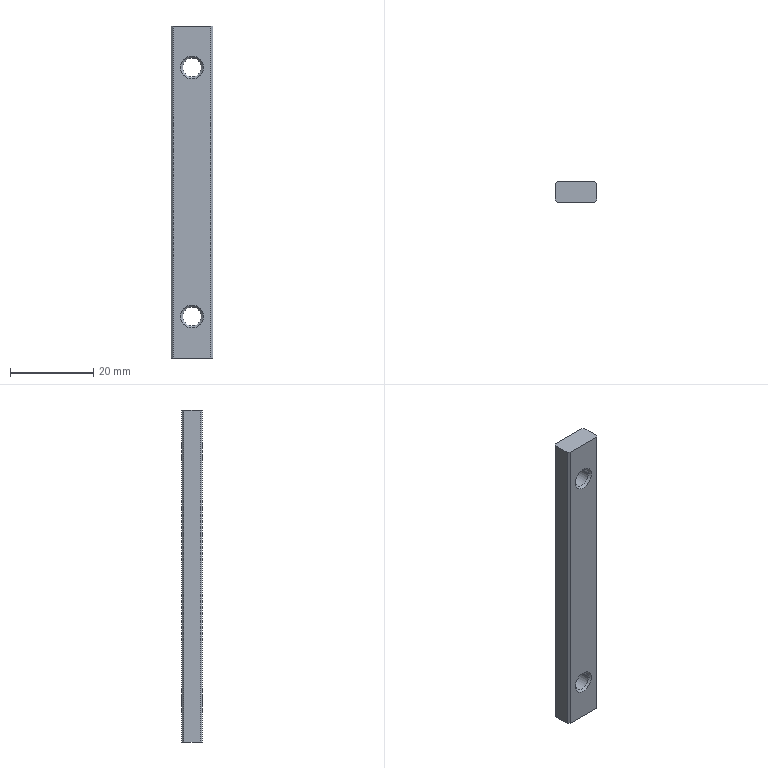Part | NX | 1 solid | 22 faces | box 10 x 5 x 80 mm | volume 3793 mm3 | plane 10 | cone 8 | cylinder 4 | commonest cylinder face diameters 4.5 x4
STEP:
#1=CARTESIAN_POINT('',(0.,2.,40.));
#2=VERTEX_POINT('',#1);
#3=CARTESIAN_POINT('',(0.,-2.,40.));
#4=VERTEX_POINT('',#3);
#5=CARTESIAN_POINT('',(0.,0.,40.));
#6=DIRECTION('',(0.,-1.,0.));
#7=VECTOR('',#6,1000.);
#8=LINE('',#5,#7);
#9=EDGE_CURVE('',#2,#4,#8,.T.);
#10=ORIENTED_EDGE('',*,*,#9,.F.);
#11=CARTESIAN_POINT('',(0.,2.,-40.));
#12=VERTEX_POINT('',#11);
#13=CARTESIAN_POINT('',(0.,2.,0.));
#14=DIRECTION('',(0.,0.,-1.));
#15=VECTOR('',#14,1000.);
#16=LINE('',#13,#15);
#17=EDGE_CURVE('',#2,#12,#16,.T.);
#18=ORIENTED_EDGE('',*,*,#17,.T.);
#19=CARTESIAN_POINT('',(0.,-2.,-40.));
#20=VERTEX_POINT('',#19);
#21=CARTESIAN_POINT('',(0.,0.,-40.));
#22=DIRECTION('',(0.,-1.,0.));
#23=VECTOR('',#22,1000.);
#24=LINE('',#21,#23);
#25=EDGE_CURVE('',#12,#20,#24,.T.);
#26=ORIENTED_EDGE('',*,*,#25,.T.);
#27=CARTESIAN_POINT('',(0.,-2.,0.));
#28=DIRECTION('',(0.,0.,1.));
#29=VECTOR('',#28,1000.);
#30=LINE('',#27,#29);
#31=EDGE_CURVE('',#20,#4,#30,.T.);
#32=ORIENTED_EDGE('',*,*,#31,.T.);
#33=EDGE_LOOP('',(#10,#18,#26,#32));
#34=FACE_BOUND('',#33,.T.);
#35=CARTESIAN_POINT('',(0.,0.,0.));
#36=DIRECTION('',(1.,0.,0.));
#37=DIRECTION('',(0.,1.,0.));
#38=AXIS2_PLACEMENT_3D('',#35,#36,#37);
#39=PLANE('',#38);
#40=ADVANCED_FACE('',(#34),#39,.F.);
#41=CARTESIAN_POINT('',(7.25,2.,-30.));
#42=VERTEX_POINT('',#41);
#43=CARTESIAN_POINT('',(2.75,2.,-30.));
#44=VERTEX_POINT('',#43);
#45=CARTESIAN_POINT('',(5.,2.,-30.));
#46=DIRECTION('',(0.,1.,0.));
#47=DIRECTION('',(1.,0.,0.));
#48=AXIS2_PLACEMENT_3D('',#45,#46,#47);
#49=CIRCLE('',#48,2.25);
#50=EDGE_CURVE('',#42,#44,#49,.T.);
#51=ORIENTED_EDGE('',*,*,#50,.T.);
#52=CARTESIAN_POINT('',(2.75,-2.,-30.));
#53=VERTEX_POINT('',#52);
#54=CARTESIAN_POINT('',(2.75,2.5,-30.));
#55=DIRECTION('',(0.,-1.,0.));
#56=VECTOR('',#55,1000.);
#57=LINE('',#54,#56);
#58=EDGE_CURVE('',#53,#44,#57,.F.);
#59=ORIENTED_EDGE('',*,*,#58,.F.);
#60=CARTESIAN_POINT('',(7.25,-2.,-30.));
#61=VERTEX_POINT('',#60);
#62=CARTESIAN_POINT('',(5.,-2.,-30.));
#63=DIRECTION('',(0.,-1.,0.));
#64=DIRECTION('',(-1.,0.,0.));
#65=AXIS2_PLACEMENT_3D('',#62,#63,#64);
#66=CIRCLE('',#65,2.25);
#67=EDGE_CURVE('',#53,#61,#66,.T.);
#68=ORIENTED_EDGE('',*,*,#67,.T.);
#69=CARTESIAN_POINT('',(7.25,2.5,-30.));
#70=DIRECTION('',(0.,-1.,0.));
#71=VECTOR('',#70,1000.);
#72=LINE('',#69,#71);
#73=EDGE_CURVE('',#61,#42,#72,.F.);
#74=ORIENTED_EDGE('',*,*,#73,.T.);
#75=EDGE_LOOP('',(#51,#59,#68,#74));
#76=FACE_BOUND('',#75,.T.);
#77=CARTESIAN_POINT('',(5.,2.5,-30.));
#78=DIRECTION('',(0.,-1.,0.));
#79=DIRECTION('',(1.,0.,0.));
#80=AXIS2_PLACEMENT_3D('',#77,#78,#79);
#81=CYLINDRICAL_SURFACE('',#80,2.25);
#82=ADVANCED_FACE('',(#76),#81,.F.);
#83=CARTESIAN_POINT('',(0.5,2.5,40.));
#84=VERTEX_POINT('',#83);
#85=CARTESIAN_POINT('',(-2.,0.,40.));
#86=DIRECTION('',(0.7071,0.7071,0.));
#87=VECTOR('',#86,1000.);
#88=LINE('',#85,#87);
#89=EDGE_CURVE('',#2,#84,#88,.T.);
#90=ORIENTED_EDGE('',*,*,#89,.T.);
#91=CARTESIAN_POINT('',(0.5,2.5,-40.));
#92=VERTEX_POINT('',#91);
#93=CARTESIAN_POINT('',(0.5,2.5,0.));
#94=DIRECTION('',(0.,0.,-1.));
#95=VECTOR('',#94,1000.);
#96=LINE('',#93,#95);
#97=EDGE_CURVE('',#84,#92,#96,.T.);
#98=ORIENTED_EDGE('',*,*,#97,.T.);
#99=CARTESIAN_POINT('',(-2.,0.,-40.));
#100=DIRECTION('',(-0.7071,-0.7071,0.));
#101=VECTOR('',#100,1000.);
#102=LINE('',#99,#101);
#103=EDGE_CURVE('',#92,#12,#102,.T.);
#104=ORIENTED_EDGE('',*,*,#103,.T.);
#105=ORIENTED_EDGE('',*,*,#17,.F.);
#106=EDGE_LOOP('',(#90,#98,#104,#105));
#107=FACE_BOUND('',#106,.T.);
#108=CARTESIAN_POINT('',(0.,2.,-40.));
#109=DIRECTION('',(-0.7071,0.7071,0.));
#110=DIRECTION('',(0.,0.,1.));
#111=AXIS2_PLACEMENT_3D('',#108,#109,#110);
#112=PLANE('',#111);
#113=ADVANCED_FACE('',(#107),#112,.T.);
#114=ORIENTED_EDGE('',*,*,#9,.T.);
#115=CARTESIAN_POINT('',(0.5,-2.5,40.));
#116=VERTEX_POINT('',#115);
#117=CARTESIAN_POINT('',(-2.,0.,40.));
#118=DIRECTION('',(-0.7071,0.7071,0.));
#119=VECTOR('',#118,1000.);
#120=LINE('',#117,#119);
#121=EDGE_CURVE('',#116,#4,#120,.T.);
#122=ORIENTED_EDGE('',*,*,#121,.F.);
#123=CARTESIAN_POINT('',(9.5,-2.5,40.));
#124=VERTEX_POINT('',#123);
#125=CARTESIAN_POINT('',(0.,-2.5,40.));
#126=DIRECTION('',(-1.,0.,0.));
#127=VECTOR('',#126,1000.);
#128=LINE('',#125,#127);
#129=EDGE_CURVE('',#124,#116,#128,.T.);
#130=ORIENTED_EDGE('',*,*,#129,.F.);
#131=CARTESIAN_POINT('',(10.,-2.,40.));
#132=VERTEX_POINT('',#131);
#133=CARTESIAN_POINT('',(12.,0.,40.));
#134=DIRECTION('',(0.7071,0.7071,0.));
#135=VECTOR('',#134,1000.);
#136=LINE('',#133,#135);
#137=EDGE_CURVE('',#124,#132,#136,.T.);
#138=ORIENTED_EDGE('',*,*,#137,.T.);
#139=CARTESIAN_POINT('',(10.,2.,40.));
#140=VERTEX_POINT('',#139);
#141=CARTESIAN_POINT('',(10.,0.,40.));
#142=DIRECTION('',(0.,-1.,0.));
#143=VECTOR('',#142,1000.);
#144=LINE('',#141,#143);
#145=EDGE_CURVE('',#140,#132,#144,.T.);
#146=ORIENTED_EDGE('',*,*,#145,.F.);
#147=CARTESIAN_POINT('',(9.5,2.5,40.));
#148=VERTEX_POINT('',#147);
#149=CARTESIAN_POINT('',(12.,0.,40.));
#150=DIRECTION('',(-0.7071,0.7071,0.));
#151=VECTOR('',#150,1000.);
#152=LINE('',#149,#151);
#153=EDGE_CURVE('',#140,#148,#152,.T.);
#154=ORIENTED_EDGE('',*,*,#153,.T.);
#155=CARTESIAN_POINT('',(0.,2.5,40.));
#156=DIRECTION('',(-1.,0.,0.));
#157=VECTOR('',#156,1000.);
#158=LINE('',#155,#157);
#159=EDGE_CURVE('',#148,#84,#158,.T.);
#160=ORIENTED_EDGE('',*,*,#159,.T.);
#161=ORIENTED_EDGE('',*,*,#89,.F.);
#162=EDGE_LOOP('',(#114,#122,#130,#138,#146,#154,#160,#161));
#163=FACE_BOUND('',#162,.T.);
#164=CARTESIAN_POINT('',(0.,2.5,40.));
#165=DIRECTION('',(0.,0.,1.));
#166=DIRECTION('',(1.,0.,0.));
#167=AXIS2_PLACEMENT_3D('',#164,#165,#166);
#168=PLANE('',#167);
#169=ADVANCED_FACE('',(#163),#168,.T.);
#170=CARTESIAN_POINT('',(0.5,-2.5,-40.));
#171=VERTEX_POINT('',#170);
#172=CARTESIAN_POINT('',(-2.,0.,-40.));
#173=DIRECTION('',(-0.7071,0.7071,0.));
#174=VECTOR('',#173,1000.);
#175=LINE('',#172,#174);
#176=EDGE_CURVE('',#171,#20,#175,.T.);
#177=ORIENTED_EDGE('',*,*,#176,.F.);
#178=CARTESIAN_POINT('',(0.5,-2.5,0.));
#179=DIRECTION('',(0.,0.,-1.));
#180=VECTOR('',#179,1000.);
#181=LINE('',#178,#180);
#182=EDGE_CURVE('',#116,#171,#181,.T.);
#183=ORIENTED_EDGE('',*,*,#182,.F.);
#184=ORIENTED_EDGE('',*,*,#121,.T.);
#185=ORIENTED_EDGE('',*,*,#31,.F.);
#186=EDGE_LOOP('',(#177,#183,#184,#185));
#187=FACE_BOUND('',#186,.T.);
#188=CARTESIAN_POINT('',(0.,-2.,39.5));
#189=DIRECTION('',(-0.7071,-0.7071,0.));
#190=DIRECTION('',(-0.7071,0.7071,0.));
#191=AXIS2_PLACEMENT_3D('',#188,#189,#190);
#192=PLANE('',#191);
#193=ADVANCED_FACE('',(#187),#192,.T.);
#194=CARTESIAN_POINT('',(10.,2.,-40.));
#195=VERTEX_POINT('',#194);
#196=CARTESIAN_POINT('',(9.5,2.5,-40.));
#197=VERTEX_POINT('',#196);
#198=CARTESIAN_POINT('',(12.,0.,-40.));
#199=DIRECTION('',(-0.7071,0.7071,0.));
#200=VECTOR('',#199,1000.);
#201=LINE('',#198,#200);
#202=EDGE_CURVE('',#195,#197,#201,.T.);
#203=ORIENTED_EDGE('',*,*,#202,.T.);
#204=CARTESIAN_POINT('',(9.5,2.5,0.));
#205=DIRECTION('',(0.,0.,-1.));
#206=VECTOR('',#205,1000.);
#207=LINE('',#204,#206);
#208=EDGE_CURVE('',#148,#197,#207,.T.);
#209=ORIENTED_EDGE('',*,*,#208,.F.);
#210=ORIENTED_EDGE('',*,*,#153,.F.);
#211=CARTESIAN_POINT('',(10.,2.,0.));
#212=DIRECTION('',(0.,0.,-1.));
#213=VECTOR('',#212,1000.);
#214=LINE('',#211,#213);
#215=EDGE_CURVE('',#140,#195,#214,.T.);
#216=ORIENTED_EDGE('',*,*,#215,.T.);
#217=EDGE_LOOP('',(#203,#209,#210,#216));
#218=FACE_BOUND('',#217,.T.);
#219=CARTESIAN_POINT('',(10.,2.,-40.));
#220=DIRECTION('',(-0.7071,-0.7071,0.));
#221=DIRECTION('',(-0.7071,0.7071,0.));
#222=AXIS2_PLACEMENT_3D('',#219,#220,#221);
#223=PLANE('',#222);
#224=ADVANCED_FACE('',(#218),#223,.F.);
#225=ORIENTED_EDGE('',*,*,#129,.T.);
#226=ORIENTED_EDGE('',*,*,#182,.T.);
#227=CARTESIAN_POINT('',(9.5,-2.5,-40.));
#228=VERTEX_POINT('',#227);
#229=CARTESIAN_POINT('',(0.,-2.5,-40.));
#230=DIRECTION('',(1.,0.,0.));
#231=VECTOR('',#230,1000.);
#232=LINE('',#229,#231);
#233=EDGE_CURVE('',#171,#228,#232,.T.);
#234=ORIENTED_EDGE('',*,*,#233,.T.);
#235=CARTESIAN_POINT('',(9.5,-2.5,0.));
#236=DIRECTION('',(0.,0.,-1.));
#237=VECTOR('',#236,1000.);
#238=LINE('',#235,#237);
#239=EDGE_CURVE('',#124,#228,#238,.T.);
#240=ORIENTED_EDGE('',*,*,#239,.F.);
#241=EDGE_LOOP('',(#225,#226,#234,#240));
#242=FACE_BOUND('',#241,.T.);
#243=CARTESIAN_POINT('',(2.25,-2.5,30.));
#244=VERTEX_POINT('',#243);
#245=CARTESIAN_POINT('',(7.75,-2.5,30.));
#246=VERTEX_POINT('',#245);
#247=CARTESIAN_POINT('',(5.,-2.5,30.));
#248=DIRECTION('',(0.,-1.,0.));
#249=DIRECTION('',(-1.,0.,0.));
#250=AXIS2_PLACEMENT_3D('',#247,#248,#249);
#251=CIRCLE('',#250,2.75);
#252=EDGE_CURVE('',#244,#246,#251,.T.);
#253=ORIENTED_EDGE('',*,*,#252,.F.);
#254=CARTESIAN_POINT('',(5.,-2.5,30.));
#255=DIRECTION('',(0.,-1.,0.));
#256=DIRECTION('',(-1.,0.,0.));
#257=AXIS2_PLACEMENT_3D('',#254,#255,#256);
#258=CIRCLE('',#257,2.75);
#259=EDGE_CURVE('',#246,#244,#258,.T.);
#260=ORIENTED_EDGE('',*,*,#259,.F.);
#261=EDGE_LOOP('',(#253,#260));
#262=FACE_BOUND('',#261,.T.);
#263=CARTESIAN_POINT('',(7.75,-2.5,-30.));
#264=VERTEX_POINT('',#263);
#265=CARTESIAN_POINT('',(2.25,-2.5,-30.));
#266=VERTEX_POINT('',#265);
#267=CARTESIAN_POINT('',(5.,-2.5,-30.));
#268=DIRECTION('',(0.,-1.,0.));
#269=DIRECTION('',(-1.,0.,0.));
#270=AXIS2_PLACEMENT_3D('',#267,#268,#269);
#271=CIRCLE('',#270,2.75);
#272=EDGE_CURVE('',#264,#266,#271,.T.);
#273=ORIENTED_EDGE('',*,*,#272,.F.);
#274=CARTESIAN_POINT('',(5.,-2.5,-30.));
#275=DIRECTION('',(0.,-1.,0.));
#276=DIRECTION('',(-1.,0.,0.));
#277=AXIS2_PLACEMENT_3D('',#274,#275,#276);
#278=CIRCLE('',#277,2.75);
#279=EDGE_CURVE('',#266,#264,#278,.T.);
#280=ORIENTED_EDGE('',*,*,#279,.F.);
#281=EDGE_LOOP('',(#273,#280));
#282=FACE_BOUND('',#281,.T.);
#283=CARTESIAN_POINT('',(0.,-2.5,40.));
#284=DIRECTION('',(0.,-1.,0.));
#285=DIRECTION('',(0.,0.,-1.));
#286=AXIS2_PLACEMENT_3D('',#283,#284,#285);
#287=PLANE('',#286);
#288=ADVANCED_FACE('',(#242,#262,#282),#287,.T.);
#289=ORIENTED_EDGE('',*,*,#137,.F.);
#290=ORIENTED_EDGE('',*,*,#239,.T.);
#291=CARTESIAN_POINT('',(10.,-2.,-40.));
#292=VERTEX_POINT('',#291);
#293=CARTESIAN_POINT('',(12.,0.,-40.));
#294=DIRECTION('',(0.7071,0.7071,0.));
#295=VECTOR('',#294,1000.);
#296=LINE('',#293,#295);
#297=EDGE_CURVE('',#228,#292,#296,.T.);
#298=ORIENTED_EDGE('',*,*,#297,.T.);
#299=CARTESIAN_POINT('',(10.,-2.,0.));
#300=DIRECTION('',(0.,0.,-1.));
#301=VECTOR('',#300,1000.);
#302=LINE('',#299,#301);
#303=EDGE_CURVE('',#132,#292,#302,.T.);
#304=ORIENTED_EDGE('',*,*,#303,.F.);
#305=EDGE_LOOP('',(#289,#290,#298,#304));
#306=FACE_BOUND('',#305,.T.);
#307=CARTESIAN_POINT('',(10.,-2.,40.));
#308=DIRECTION('',(-0.7071,0.7071,0.));
#309=DIRECTION('',(0.,0.,1.));
#310=AXIS2_PLACEMENT_3D('',#307,#308,#309);
#311=PLANE('',#310);
#312=ADVANCED_FACE('',(#306),#311,.F.);
#313=CARTESIAN_POINT('',(10.,0.,-40.));
#314=DIRECTION('',(0.,-1.,0.));
#315=VECTOR('',#314,1000.);
#316=LINE('',#313,#315);
#317=EDGE_CURVE('',#195,#292,#316,.T.);
#318=ORIENTED_EDGE('',*,*,#317,.F.);
#319=ORIENTED_EDGE('',*,*,#215,.F.);
#320=ORIENTED_EDGE('',*,*,#145,.T.);
#321=ORIENTED_EDGE('',*,*,#303,.T.);
#322=EDGE_LOOP('',(#318,#319,#320,#321));
#323=FACE_BOUND('',#322,.T.);
#324=CARTESIAN_POINT('',(10.,0.,0.));
#325=DIRECTION('',(1.,0.,0.));
#326=DIRECTION('',(0.,1.,0.));
#327=AXIS2_PLACEMENT_3D('',#324,#325,#326);
#328=PLANE('',#327);
#329=ADVANCED_FACE('',(#323),#328,.T.);
#330=CARTESIAN_POINT('',(2.75,-2.,30.));
#331=VERTEX_POINT('',#330);
#332=CARTESIAN_POINT('',(7.25,-2.,30.));
#333=VERTEX_POINT('',#332);
#334=CARTESIAN_POINT('',(5.,-2.,30.));
#335=DIRECTION('',(0.,-1.,0.));
#336=DIRECTION('',(-1.,0.,0.));
#337=AXIS2_PLACEMENT_3D('',#334,#335,#336);
#338=CIRCLE('',#337,2.25);
#339=EDGE_CURVE('',#331,#333,#338,.T.);
#340=ORIENTED_EDGE('',*,*,#339,.T.);
#341=CARTESIAN_POINT('',(7.25,2.,30.));
#342=VERTEX_POINT('',#341);
#343=CARTESIAN_POINT('',(7.25,2.5,30.));
#344=DIRECTION('',(0.,-1.,0.));
#345=VECTOR('',#344,1000.);
#346=LINE('',#343,#345);
#347=EDGE_CURVE('',#342,#333,#346,.T.);
#348=ORIENTED_EDGE('',*,*,#347,.F.);
#349=CARTESIAN_POINT('',(2.75,2.,30.));
#350=VERTEX_POINT('',#349);
#351=CARTESIAN_POINT('',(5.,2.,30.));
#352=DIRECTION('',(0.,1.,0.));
#353=DIRECTION('',(1.,0.,0.));
#354=AXIS2_PLACEMENT_3D('',#351,#352,#353);
#355=CIRCLE('',#354,2.25);
#356=EDGE_CURVE('',#342,#350,#355,.T.);
#357=ORIENTED_EDGE('',*,*,#356,.T.);
#358=CARTESIAN_POINT('',(2.75,2.5,30.));
#359=DIRECTION('',(0.,-1.,0.));
#360=VECTOR('',#359,1000.);
#361=LINE('',#358,#360);
#362=EDGE_CURVE('',#350,#331,#361,.T.);
#363=ORIENTED_EDGE('',*,*,#362,.T.);
#364=EDGE_LOOP('',(#340,#348,#357,#363));
#365=FACE_BOUND('',#364,.T.);
#366=CARTESIAN_POINT('',(5.,2.5,30.));
#367=DIRECTION('',(0.,-1.,0.));
#368=DIRECTION('',(1.,0.,0.));
#369=AXIS2_PLACEMENT_3D('',#366,#367,#368);
#370=CYLINDRICAL_SURFACE('',#369,2.25);
#371=ADVANCED_FACE('',(#365),#370,.F.);
#372=CARTESIAN_POINT('',(0.,2.5,-40.));
#373=DIRECTION('',(1.,0.,0.));
#374=VECTOR('',#373,1000.);
#375=LINE('',#372,#374);
#376=EDGE_CURVE('',#92,#197,#375,.T.);
#377=ORIENTED_EDGE('',*,*,#376,.F.);
#378=ORIENTED_EDGE('',*,*,#97,.F.);
#379=ORIENTED_EDGE('',*,*,#159,.F.);
#380=ORIENTED_EDGE('',*,*,#208,.T.);
#381=EDGE_LOOP('',(#377,#378,#379,#380));
#382=FACE_BOUND('',#381,.T.);
#383=CARTESIAN_POINT('',(7.75,2.5,30.));
#384=VERTEX_POINT('',#383);
#385=CARTESIAN_POINT('',(2.25,2.5,30.));
#386=VERTEX_POINT('',#385);
#387=CARTESIAN_POINT('',(5.,2.5,30.));
#388=DIRECTION('',(0.,1.,0.));
#389=DIRECTION('',(1.,0.,0.));
#390=AXIS2_PLACEMENT_3D('',#387,#388,#389);
#391=CIRCLE('',#390,2.75);
#392=EDGE_CURVE('',#384,#386,#391,.T.);
#393=ORIENTED_EDGE('',*,*,#392,.F.);
#394=CARTESIAN_POINT('',(5.,2.5,30.));
#395=DIRECTION('',(0.,1.,0.));
#396=DIRECTION('',(1.,0.,0.));
#397=AXIS2_PLACEMENT_3D('',#394,#395,#396);
#398=CIRCLE('',#397,2.75);
#399=EDGE_CURVE('',#386,#384,#398,.T.);
#400=ORIENTED_EDGE('',*,*,#399,.F.);
#401=EDGE_LOOP('',(#393,#400));
#402=FACE_BOUND('',#401,.T.);
#403=CARTESIAN_POINT('',(2.25,2.5,-30.));
#404=VERTEX_POINT('',#403);
#405=CARTESIAN_POINT('',(7.75,2.5,-30.));
#406=VERTEX_POINT('',#405);
#407=CARTESIAN_POINT('',(5.,2.5,-30.));
#408=DIRECTION('',(0.,1.,0.));
#409=DIRECTION('',(1.,0.,0.));
#410=AXIS2_PLACEMENT_3D('',#407,#408,#409);
#411=CIRCLE('',#410,2.75);
#412=EDGE_CURVE('',#404,#406,#411,.T.);
#413=ORIENTED_EDGE('',*,*,#412,.F.);
#414=CARTESIAN_POINT('',(5.,2.5,-30.));
#415=DIRECTION('',(0.,1.,0.));
#416=DIRECTION('',(1.,0.,0.));
#417=AXIS2_PLACEMENT_3D('',#414,#415,#416);
#418=CIRCLE('',#417,2.75);
#419=EDGE_CURVE('',#406,#404,#418,.T.);
#420=ORIENTED_EDGE('',*,*,#419,.F.);
#421=EDGE_LOOP('',(#413,#420));
#422=FACE_BOUND('',#421,.T.);
#423=CARTESIAN_POINT('',(0.,2.5,-40.));
#424=DIRECTION('',(0.,1.,0.));
#425=DIRECTION('',(1.,0.,0.));
#426=AXIS2_PLACEMENT_3D('',#423,#424,#425);
#427=PLANE('',#426);
#428=ADVANCED_FACE('',(#382,#402,#422),#427,.T.);
#429=ORIENTED_EDGE('',*,*,#176,.T.);
#430=ORIENTED_EDGE('',*,*,#25,.F.);
#431=ORIENTED_EDGE('',*,*,#103,.F.);
#432=ORIENTED_EDGE('',*,*,#376,.T.);
#433=ORIENTED_EDGE('',*,*,#202,.F.);
#434=ORIENTED_EDGE('',*,*,#317,.T.);
#435=ORIENTED_EDGE('',*,*,#297,.F.);
#436=ORIENTED_EDGE('',*,*,#233,.F.);
#437=EDGE_LOOP('',(#429,#430,#431,#432,#433,#434,#435,#436));
#438=FACE_BOUND('',#437,.T.);
#439=CARTESIAN_POINT('',(0.,-2.5,-40.));
#440=DIRECTION('',(0.,0.,-1.));
#441=DIRECTION('',(0.,-1.,0.));
#442=AXIS2_PLACEMENT_3D('',#439,#440,#441);
#443=PLANE('',#442);
#444=ADVANCED_FACE('',(#438),#443,.T.);
#445=ORIENTED_EDGE('',*,*,#412,.T.);
#446=CARTESIAN_POINT('',(7.75,2.5,-30.));
#447=DIRECTION('',(0.7071,0.7071,0.));
#448=VECTOR('',#447,1000.);
#449=LINE('',#446,#448);
#450=EDGE_CURVE('',#42,#406,#449,.T.);
#451=ORIENTED_EDGE('',*,*,#450,.F.);
#452=CARTESIAN_POINT('',(5.,2.,-30.));
#453=DIRECTION('',(0.,1.,0.));
#454=DIRECTION('',(1.,0.,0.));
#455=AXIS2_PLACEMENT_3D('',#452,#453,#454);
#456=CIRCLE('',#455,2.25);
#457=EDGE_CURVE('',#44,#42,#456,.T.);
#458=ORIENTED_EDGE('',*,*,#457,.F.);
#459=CARTESIAN_POINT('',(2.25,2.5,-30.));
#460=DIRECTION('',(-0.7071,0.7071,0.));
#461=VECTOR('',#460,1000.);
#462=LINE('',#459,#461);
#463=EDGE_CURVE('',#44,#404,#462,.T.);
#464=ORIENTED_EDGE('',*,*,#463,.T.);
#465=EDGE_LOOP('',(#445,#451,#458,#464));
#466=FACE_BOUND('',#465,.T.);
#467=CARTESIAN_POINT('',(5.,2.5,-30.));
#468=DIRECTION('',(0.,1.,0.));
#469=DIRECTION('',(1.,0.,0.));
#470=AXIS2_PLACEMENT_3D('',#467,#468,#469);
#471=CONICAL_SURFACE('',#470,2.75,0.7854);
#472=ADVANCED_FACE('',(#466),#471,.F.);
#473=ORIENTED_EDGE('',*,*,#392,.T.);
#474=CARTESIAN_POINT('',(2.25,2.5,30.));
#475=DIRECTION('',(-0.7071,0.7071,0.));
#476=VECTOR('',#475,1000.);
#477=LINE('',#474,#476);
#478=EDGE_CURVE('',#386,#350,#477,.F.);
#479=ORIENTED_EDGE('',*,*,#478,.T.);
#480=ORIENTED_EDGE('',*,*,#356,.F.);
#481=CARTESIAN_POINT('',(7.75,2.5,30.));
#482=DIRECTION('',(0.7071,0.7071,0.));
#483=VECTOR('',#482,1000.);
#484=LINE('',#481,#483);
#485=EDGE_CURVE('',#384,#342,#484,.F.);
#486=ORIENTED_EDGE('',*,*,#485,.F.);
#487=EDGE_LOOP('',(#473,#479,#480,#486));
#488=FACE_BOUND('',#487,.T.);
#489=CARTESIAN_POINT('',(5.,2.5,30.));
#490=DIRECTION('',(0.,1.,0.));
#491=DIRECTION('',(1.,0.,0.));
#492=AXIS2_PLACEMENT_3D('',#489,#490,#491);
#493=CONICAL_SURFACE('',#492,2.75,0.7854);
#494=ADVANCED_FACE('',(#488),#493,.F.);
#495=ORIENTED_EDGE('',*,*,#272,.T.);
#496=CARTESIAN_POINT('',(2.25,-2.5,-30.));
#497=DIRECTION('',(-0.7071,-0.7071,0.));
#498=VECTOR('',#497,1000.);
#499=LINE('',#496,#498);
#500=EDGE_CURVE('',#266,#53,#499,.F.);
#501=ORIENTED_EDGE('',*,*,#500,.T.);
#502=CARTESIAN_POINT('',(5.,-2.,-30.));
#503=DIRECTION('',(0.,-1.,0.));
#504=DIRECTION('',(-1.,0.,0.));
#505=AXIS2_PLACEMENT_3D('',#502,#503,#504);
#506=CIRCLE('',#505,2.25);
#507=EDGE_CURVE('',#61,#53,#506,.T.);
#508=ORIENTED_EDGE('',*,*,#507,.F.);
#509=CARTESIAN_POINT('',(7.75,-2.5,-30.));
#510=DIRECTION('',(0.7071,-0.7071,0.));
#511=VECTOR('',#510,1000.);
#512=LINE('',#509,#511);
#513=EDGE_CURVE('',#264,#61,#512,.F.);
#514=ORIENTED_EDGE('',*,*,#513,.F.);
#515=EDGE_LOOP('',(#495,#501,#508,#514));
#516=FACE_BOUND('',#515,.T.);
#517=CARTESIAN_POINT('',(5.,-2.5,-30.));
#518=DIRECTION('',(0.,-1.,0.));
#519=DIRECTION('',(-1.,0.,0.));
#520=AXIS2_PLACEMENT_3D('',#517,#518,#519);
#521=CONICAL_SURFACE('',#520,2.75,0.7854);
#522=ADVANCED_FACE('',(#516),#521,.F.);
#523=ORIENTED_EDGE('',*,*,#252,.T.);
#524=CARTESIAN_POINT('',(7.75,-2.5,30.));
#525=DIRECTION('',(0.7071,-0.7071,0.));
#526=VECTOR('',#525,1000.);
#527=LINE('',#524,#526);
#528=EDGE_CURVE('',#246,#333,#527,.F.);
#529=ORIENTED_EDGE('',*,*,#528,.T.);
#530=ORIENTED_EDGE('',*,*,#339,.F.);
#531=CARTESIAN_POINT('',(2.25,-2.5,30.));
#532=DIRECTION('',(-0.7071,-0.7071,0.));
#533=VECTOR('',#532,1000.);
#534=LINE('',#531,#533);
#535=EDGE_CURVE('',#244,#331,#534,.F.);
#536=ORIENTED_EDGE('',*,*,#535,.F.);
#537=EDGE_LOOP('',(#523,#529,#530,#536));
#538=FACE_BOUND('',#537,.T.);
#539=CARTESIAN_POINT('',(5.,-2.5,30.));
#540=DIRECTION('',(0.,-1.,0.));
#541=DIRECTION('',(-1.,0.,0.));
#542=AXIS2_PLACEMENT_3D('',#539,#540,#541);
#543=CONICAL_SURFACE('',#542,2.75,0.7854);
#544=ADVANCED_FACE('',(#538),#543,.F.);
#545=CARTESIAN_POINT('',(5.,2.,30.));
#546=DIRECTION('',(0.,1.,0.));
#547=DIRECTION('',(1.,0.,0.));
#548=AXIS2_PLACEMENT_3D('',#545,#546,#547);
#549=CIRCLE('',#548,2.25);
#550=EDGE_CURVE('',#350,#342,#549,.T.);
#551=ORIENTED_EDGE('',*,*,#550,.F.);
#552=ORIENTED_EDGE('',*,*,#478,.F.);
#553=ORIENTED_EDGE('',*,*,#399,.T.);
#554=ORIENTED_EDGE('',*,*,#485,.T.);
#555=EDGE_LOOP('',(#551,#552,#553,#554));
#556=FACE_BOUND('',#555,.T.);
#557=CARTESIAN_POINT('',(5.,2.5,30.));
#558=DIRECTION('',(0.,1.,0.));
#559=DIRECTION('',(1.,0.,0.));
#560=AXIS2_PLACEMENT_3D('',#557,#558,#559);
#561=CONICAL_SURFACE('',#560,2.75,0.7854);
#562=ADVANCED_FACE('',(#556),#561,.F.);
#563=ORIENTED_EDGE('',*,*,#550,.T.);
#564=ORIENTED_EDGE('',*,*,#347,.T.);
#565=CARTESIAN_POINT('',(5.,-2.,30.));
#566=DIRECTION('',(0.,-1.,0.));
#567=DIRECTION('',(-1.,0.,0.));
#568=AXIS2_PLACEMENT_3D('',#565,#566,#567);
#569=CIRCLE('',#568,2.25);
#570=EDGE_CURVE('',#333,#331,#569,.T.);
#571=ORIENTED_EDGE('',*,*,#570,.T.);
#572=ORIENTED_EDGE('',*,*,#362,.F.);
#573=EDGE_LOOP('',(#563,#564,#571,#572));
#574=FACE_BOUND('',#573,.T.);
#575=CARTESIAN_POINT('',(5.,2.5,30.));
#576=DIRECTION('',(0.,-1.,0.));
#577=DIRECTION('',(1.,0.,0.));
#578=AXIS2_PLACEMENT_3D('',#575,#576,#577);
#579=CYLINDRICAL_SURFACE('',#578,2.25);
#580=ADVANCED_FACE('',(#574),#579,.F.);
#581=ORIENTED_EDGE('',*,*,#535,.T.);
#582=ORIENTED_EDGE('',*,*,#570,.F.);
#583=ORIENTED_EDGE('',*,*,#528,.F.);
#584=ORIENTED_EDGE('',*,*,#259,.T.);
#585=EDGE_LOOP('',(#581,#582,#583,#584));
#586=FACE_BOUND('',#585,.T.);
#587=CARTESIAN_POINT('',(5.,-2.5,30.));
#588=DIRECTION('',(0.,-1.,0.));
#589=DIRECTION('',(-1.,0.,0.));
#590=AXIS2_PLACEMENT_3D('',#587,#588,#589);
#591=CONICAL_SURFACE('',#590,2.75,0.7854);
#592=ADVANCED_FACE('',(#586),#591,.F.);
#593=ORIENTED_EDGE('',*,*,#500,.F.);
#594=ORIENTED_EDGE('',*,*,#279,.T.);
#595=ORIENTED_EDGE('',*,*,#513,.T.);
#596=ORIENTED_EDGE('',*,*,#67,.F.);
#597=EDGE_LOOP('',(#593,#594,#595,#596));
#598=FACE_BOUND('',#597,.T.);
#599=CARTESIAN_POINT('',(5.,-2.5,-30.));
#600=DIRECTION('',(0.,-1.,0.));
#601=DIRECTION('',(-1.,0.,0.));
#602=AXIS2_PLACEMENT_3D('',#599,#600,#601);
#603=CONICAL_SURFACE('',#602,2.75,0.7854);
#604=ADVANCED_FACE('',(#598),#603,.F.);
#605=ORIENTED_EDGE('',*,*,#507,.T.);
#606=ORIENTED_EDGE('',*,*,#58,.T.);
#607=ORIENTED_EDGE('',*,*,#457,.T.);
#608=ORIENTED_EDGE('',*,*,#73,.F.);
#609=EDGE_LOOP('',(#605,#606,#607,#608));
#610=FACE_BOUND('',#609,.T.);
#611=CARTESIAN_POINT('',(5.,2.5,-30.));
#612=DIRECTION('',(0.,-1.,0.));
#613=DIRECTION('',(1.,0.,0.));
#614=AXIS2_PLACEMENT_3D('',#611,#612,#613);
#615=CYLINDRICAL_SURFACE('',#614,2.25);
#616=ADVANCED_FACE('',(#610),#615,.F.);
#617=ORIENTED_EDGE('',*,*,#50,.F.);
#618=ORIENTED_EDGE('',*,*,#450,.T.);
#619=ORIENTED_EDGE('',*,*,#419,.T.);
#620=ORIENTED_EDGE('',*,*,#463,.F.);
#621=EDGE_LOOP('',(#617,#618,#619,#620));
#622=FACE_BOUND('',#621,.T.);
#623=CARTESIAN_POINT('',(5.,2.5,-30.));
#624=DIRECTION('',(0.,1.,0.));
#625=DIRECTION('',(1.,0.,0.));
#626=AXIS2_PLACEMENT_3D('',#623,#624,#625);
#627=CONICAL_SURFACE('',#626,2.75,0.7854);
#628=ADVANCED_FACE('',(#622),#627,.F.);
#629=CLOSED_SHELL('',(#40,#82,#113,#169,#193,#224,#288,#312,#329,#371,#428,#444,#472,#494,#522,#544,#562,#580,#592,#604,#616,#628));
#630=MANIFOLD_SOLID_BREP('',#629);
#631=(LENGTH_UNIT()NAMED_UNIT(*)SI_UNIT(.MILLI.,.METRE.));
#632=UNCERTAINTY_MEASURE_WITH_UNIT(LENGTH_MEASURE(0.00001),#631,'','');
#633=(NAMED_UNIT(*)PLANE_ANGLE_UNIT()SI_UNIT($,.RADIAN.));
#634=(NAMED_UNIT(*)SI_UNIT($,.STERADIAN.)SOLID_ANGLE_UNIT());
#635=(GEOMETRIC_REPRESENTATION_CONTEXT(3)GLOBAL_UNCERTAINTY_ASSIGNED_CONTEXT((#632))GLOBAL_UNIT_ASSIGNED_CONTEXT((#631,#633,#634))REPRESENTATION_CONTEXT('',''));
#636=ADVANCED_BREP_SHAPE_REPRESENTATION('',(#630),#635);